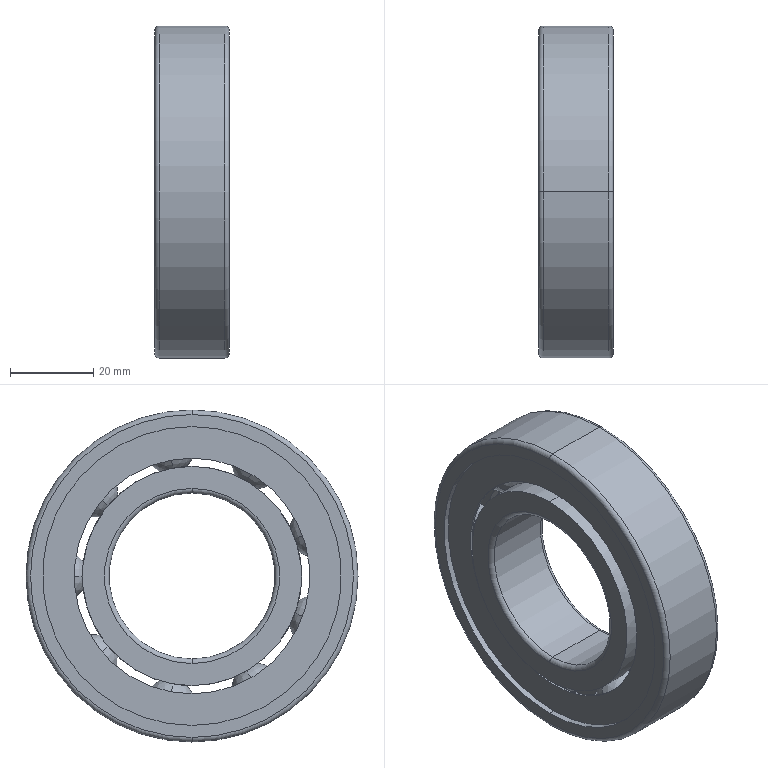Part | STEP file | GB/T276-94 deep groove ball bearing 6208-2Z | 1 solid | 160 faces | box 18 x 80 x 80 mm | volume 42698 mm3 | sphere 72 | torus 38 | plane 26 | cylinder 24 | commonest cylinder face diameters 72 x8 52.8 x4 56.76 x4 40 x2 59.1 x2 65.7 x2